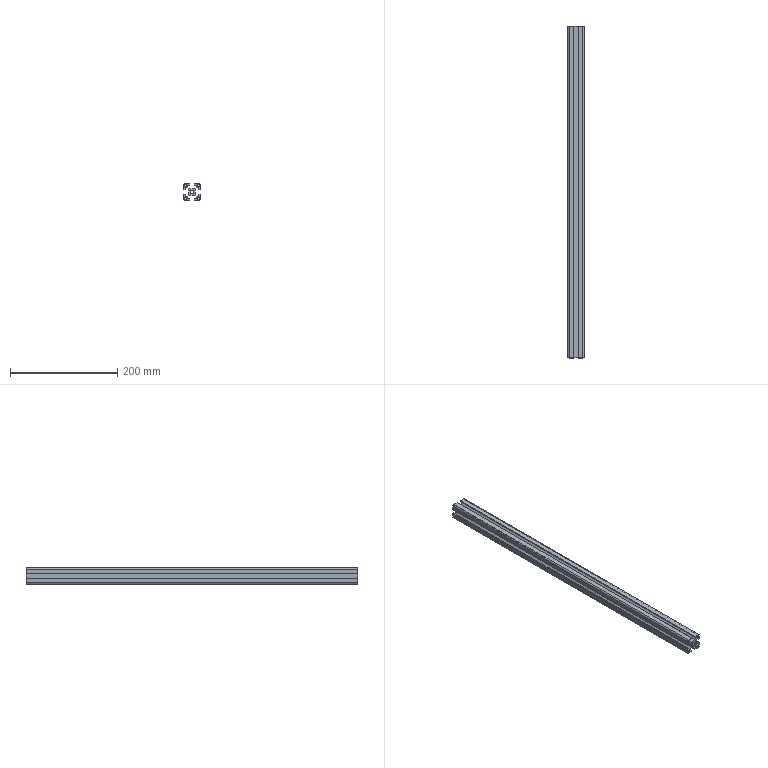Part | SolidWorks | features Extrusion 1 | 1 solid | 60 faces | box 30 x 620 x 30 mm | volume 206173 mm3 | plane 46 | cylinder 14 | commonest cylinder face diameters 4.2 x8 4 x4 6.8 x2